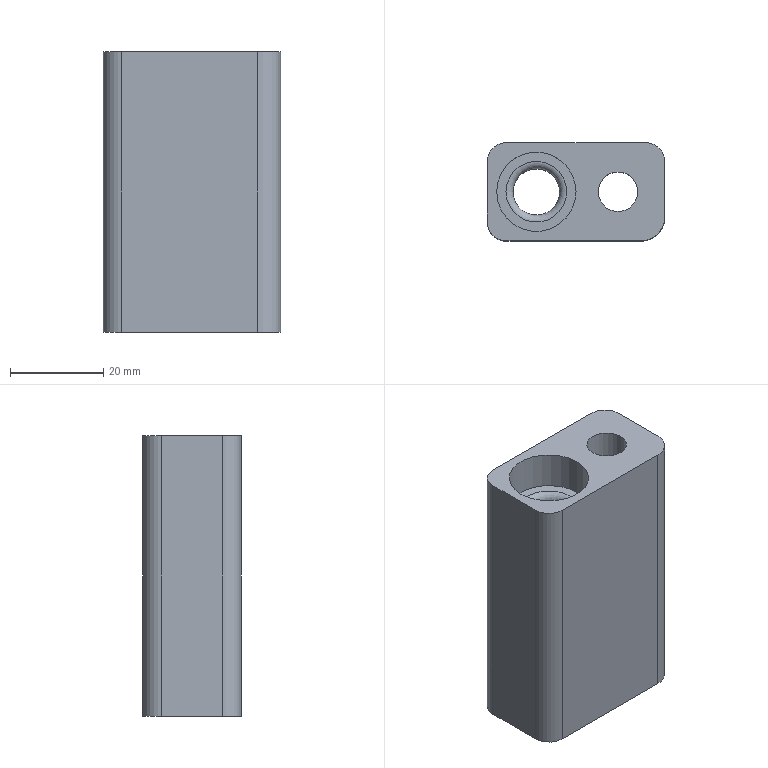Part | STEP file | gslz 2016.10.28-10_id2338_x_t | 1 solid | 17 faces | box 38 x 21 x 60 mm | volume 33724 mm3 | plane 8 | cylinder 8 | torus 1 | commonest cylinder face diameters 8 x3 10 x2 8.5 x1 14 x1 17 x1
STEP:
#1=CARTESIAN_POINT('',(0.,0.,0.));
#2=DIRECTION('',(0.,0.,1.));
#3=DIRECTION('',(1.,0.,0.));
#4=AXIS2_PLACEMENT_3D('',#1,#2,#3);
#5=CARTESIAN_POINT('',(1013.442,-82.206,85.));
#6=VERTEX_POINT('',#5);
#7=CARTESIAN_POINT('',(1021.942,-82.206,85.));
#8=DIRECTION('',(0.,0.,1.));
#9=DIRECTION('',(-1.,0.,0.));
#10=AXIS2_PLACEMENT_3D('',#7,#8,#9);
#11=CIRCLE('',#10,8.5);
#12=CARTESIAN_POINT('',(980.942,-76.206,85.));
#13=DIRECTION('',(0.,0.,1.));
#14=DIRECTION('',(1.,0.,0.));
#15=AXIS2_PLACEMENT_3D('',#12,#13,#14);
#16=PLANE('',#15);
#17=CARTESIAN_POINT('',(41.,-6.));
#18=DIRECTION('',(-1.,0.));
#19=AXIS2_PLACEMENT_2D('',#17,#18);
#20=CIRCLE('',#19,8.5);
#21=(GEOMETRIC_REPRESENTATION_CONTEXT(2)PARAMETRIC_REPRESENTATION_CONTEXT()REPRESENTATION_CONTEXT('',''));
#22=DEFINITIONAL_REPRESENTATION('',(#20),#21);
#23=PCURVE('',#16,#22);
#24=CARTESIAN_POINT('',(1021.942,-82.206,81.));
#25=DIRECTION('',(0.,0.,-1.));
#26=DIRECTION('',(1.,0.,0.));
#27=AXIS2_PLACEMENT_3D('',#24,#25,#26);
#28=CYLINDRICAL_SURFACE('',#27,8.5);
#29=CARTESIAN_POINT('',(9.425,-4.));
#30=DIRECTION('',(-1.,0.));
#31=VECTOR('',#30,1.);
#32=LINE('',#29,#31);
#33=(GEOMETRIC_REPRESENTATION_CONTEXT(2)PARAMETRIC_REPRESENTATION_CONTEXT()REPRESENTATION_CONTEXT('',''));
#34=DEFINITIONAL_REPRESENTATION('',(#32),#33);
#35=PCURVE('',#28,#34);
#36=SURFACE_CURVE('',#11,(#23,#35),.PCURVE_S1.);
#37=EDGE_CURVE('',#6,#6,#36,.T.);
#38=ORIENTED_EDGE('',*,*,#37,.F.);
#39=EDGE_LOOP('',(#38));
#40=FACE_BOUND('',#39,.T.);
#41=CARTESIAN_POINT('',(1049.442,-87.706,85.));
#42=VERTEX_POINT('',#41);
#43=CARTESIAN_POINT('',(1049.442,-75.706,85.));
#44=VERTEX_POINT('',#43);
#45=CARTESIAN_POINT('',(1049.442,-76.206,85.));
#46=DIRECTION('',(0.,1.,0.));
#47=VECTOR('',#46,1.);
#48=LINE('',#45,#47);
#49=CARTESIAN_POINT('',(68.5,0.));
#50=DIRECTION('',(0.,1.));
#51=VECTOR('',#50,1.);
#52=LINE('',#49,#51);
#53=(GEOMETRIC_REPRESENTATION_CONTEXT(2)PARAMETRIC_REPRESENTATION_CONTEXT()REPRESENTATION_CONTEXT('',''));
#54=DEFINITIONAL_REPRESENTATION('',(#52),#53);
#55=PCURVE('',#16,#54);
#56=CARTESIAN_POINT('',(1049.442,-82.206,43.5));
#57=DIRECTION('',(1.,0.,0.));
#58=DIRECTION('',(0.,0.,-1.));
#59=AXIS2_PLACEMENT_3D('',#56,#57,#58);
#60=PLANE('',#59);
#61=CARTESIAN_POINT('',(-41.5,6.));
#62=DIRECTION('',(0.,1.));
#63=VECTOR('',#62,1.);
#64=LINE('',#61,#63);
#65=(GEOMETRIC_REPRESENTATION_CONTEXT(2)PARAMETRIC_REPRESENTATION_CONTEXT()REPRESENTATION_CONTEXT('',''));
#66=DEFINITIONAL_REPRESENTATION('',(#64),#65);
#67=PCURVE('',#60,#66);
#68=SURFACE_CURVE('',#48,(#55,#67),.PCURVE_S1.);
#69=EDGE_CURVE('',#42,#44,#68,.T.);
#70=ORIENTED_EDGE('',*,*,#69,.T.);
#71=CARTESIAN_POINT('',(1045.442,-71.706,85.));
#72=VERTEX_POINT('',#71);
#73=CARTESIAN_POINT('',(1045.442,-75.706,85.));
#74=DIRECTION('',(0.,0.,1.));
#75=DIRECTION('',(-1.,0.,0.));
#76=AXIS2_PLACEMENT_3D('',#73,#74,#75);
#77=CIRCLE('',#76,4.);
#78=CARTESIAN_POINT('',(64.5,0.5));
#79=DIRECTION('',(-1.,0.));
#80=AXIS2_PLACEMENT_2D('',#78,#79);
#81=CIRCLE('',#80,4.);
#82=(GEOMETRIC_REPRESENTATION_CONTEXT(2)PARAMETRIC_REPRESENTATION_CONTEXT()REPRESENTATION_CONTEXT('',''));
#83=DEFINITIONAL_REPRESENTATION('',(#81),#82);
#84=PCURVE('',#16,#83);
#85=CARTESIAN_POINT('',(1045.442,-75.706,43.5));
#86=DIRECTION('',(0.,0.,-1.));
#87=DIRECTION('',(-1.,0.,0.));
#88=AXIS2_PLACEMENT_3D('',#85,#86,#87);
#89=CYLINDRICAL_SURFACE('',#88,4.);
#90=CARTESIAN_POINT('',(6.283,-41.5));
#91=DIRECTION('',(-1.,0.));
#92=VECTOR('',#91,1.);
#93=LINE('',#90,#92);
#94=(GEOMETRIC_REPRESENTATION_CONTEXT(2)PARAMETRIC_REPRESENTATION_CONTEXT()REPRESENTATION_CONTEXT('',''));
#95=DEFINITIONAL_REPRESENTATION('',(#93),#94);
#96=PCURVE('',#89,#95);
#97=SURFACE_CURVE('',#77,(#84,#96),.PCURVE_S1.);
#98=EDGE_CURVE('',#44,#72,#97,.T.);
#99=ORIENTED_EDGE('',*,*,#98,.T.);
#100=CARTESIAN_POINT('',(1015.442,-71.706,85.));
#101=VERTEX_POINT('',#100);
#102=CARTESIAN_POINT('',(938.307,-71.706,85.));
#103=DIRECTION('',(-1.,0.,0.));
#104=VECTOR('',#103,1.);
#105=LINE('',#102,#104);
#106=CARTESIAN_POINT('',(-42.635,4.5));
#107=DIRECTION('',(-1.,0.));
#108=VECTOR('',#107,1.);
#109=LINE('',#106,#108);
#110=(GEOMETRIC_REPRESENTATION_CONTEXT(2)PARAMETRIC_REPRESENTATION_CONTEXT()REPRESENTATION_CONTEXT('',''));
#111=DEFINITIONAL_REPRESENTATION('',(#109),#110);
#112=PCURVE('',#16,#111);
#113=CARTESIAN_POINT('',(938.307,-71.706,80.));
#114=DIRECTION('',(0.,-1.,0.));
#115=DIRECTION('',(0.,0.,-1.));
#116=AXIS2_PLACEMENT_3D('',#113,#114,#115);
#117=PLANE('',#116);
#118=CARTESIAN_POINT('',(-5.,0.));
#119=DIRECTION('',(0.,-1.));
#120=VECTOR('',#119,1.);
#121=LINE('',#118,#120);
#122=(GEOMETRIC_REPRESENTATION_CONTEXT(2)PARAMETRIC_REPRESENTATION_CONTEXT()REPRESENTATION_CONTEXT('',''));
#123=DEFINITIONAL_REPRESENTATION('',(#121),#122);
#124=PCURVE('',#117,#123);
#125=SURFACE_CURVE('',#105,(#112,#124),.PCURVE_S1.);
#126=EDGE_CURVE('',#72,#101,#125,.T.);
#127=ORIENTED_EDGE('',*,*,#126,.T.);
#128=CARTESIAN_POINT('',(1011.442,-75.706,85.));
#129=VERTEX_POINT('',#128);
#130=CARTESIAN_POINT('',(1015.442,-75.706,85.));
#131=DIRECTION('',(0.,0.,1.));
#132=DIRECTION('',(-1.,0.,0.));
#133=AXIS2_PLACEMENT_3D('',#130,#131,#132);
#134=CIRCLE('',#133,4.);
#135=CARTESIAN_POINT('',(34.5,0.5));
#136=DIRECTION('',(-1.,0.));
#137=AXIS2_PLACEMENT_2D('',#135,#136);
#138=CIRCLE('',#137,4.);
#139=(GEOMETRIC_REPRESENTATION_CONTEXT(2)PARAMETRIC_REPRESENTATION_CONTEXT()REPRESENTATION_CONTEXT('',''));
#140=DEFINITIONAL_REPRESENTATION('',(#138),#139);
#141=PCURVE('',#16,#140);
#142=CARTESIAN_POINT('',(1015.442,-75.706,46.));
#143=DIRECTION('',(0.,0.,-1.));
#144=DIRECTION('',(-1.,0.,0.));
#145=AXIS2_PLACEMENT_3D('',#142,#143,#144);
#146=CYLINDRICAL_SURFACE('',#145,4.);
#147=CARTESIAN_POINT('',(6.283,-39.));
#148=DIRECTION('',(-1.,0.));
#149=VECTOR('',#148,1.);
#150=LINE('',#147,#149);
#151=(GEOMETRIC_REPRESENTATION_CONTEXT(2)PARAMETRIC_REPRESENTATION_CONTEXT()REPRESENTATION_CONTEXT('',''));
#152=DEFINITIONAL_REPRESENTATION('',(#150),#151);
#153=PCURVE('',#146,#152);
#154=SURFACE_CURVE('',#134,(#141,#153),.PCURVE_S1.);
#155=EDGE_CURVE('',#101,#129,#154,.T.);
#156=ORIENTED_EDGE('',*,*,#155,.T.);
#157=CARTESIAN_POINT('',(1011.442,-88.706,85.));
#158=VERTEX_POINT('',#157);
#159=CARTESIAN_POINT('',(1011.442,-82.206,85.));
#160=DIRECTION('',(0.,-1.,0.));
#161=VECTOR('',#160,1.);
#162=LINE('',#159,#161);
#163=CARTESIAN_POINT('',(30.5,-6.));
#164=DIRECTION('',(0.,-1.));
#165=VECTOR('',#164,1.);
#166=LINE('',#163,#165);
#167=(GEOMETRIC_REPRESENTATION_CONTEXT(2)PARAMETRIC_REPRESENTATION_CONTEXT()REPRESENTATION_CONTEXT('',''));
#168=DEFINITIONAL_REPRESENTATION('',(#166),#167);
#169=PCURVE('',#16,#168);
#170=CARTESIAN_POINT('',(1011.442,-82.206,46.));
#171=DIRECTION('',(1.,0.,0.));
#172=DIRECTION('',(0.,0.,-1.));
#173=AXIS2_PLACEMENT_3D('',#170,#171,#172);
#174=PLANE('',#173);
#175=CARTESIAN_POINT('',(-39.,0.));
#176=DIRECTION('',(0.,-1.));
#177=VECTOR('',#176,1.);
#178=LINE('',#175,#177);
#179=(GEOMETRIC_REPRESENTATION_CONTEXT(2)PARAMETRIC_REPRESENTATION_CONTEXT()REPRESENTATION_CONTEXT('',''));
#180=DEFINITIONAL_REPRESENTATION('',(#178),#179);
#181=PCURVE('',#174,#180);
#182=SURFACE_CURVE('',#162,(#169,#181),.PCURVE_S1.);
#183=EDGE_CURVE('',#129,#158,#182,.T.);
#184=ORIENTED_EDGE('',*,*,#183,.T.);
#185=CARTESIAN_POINT('',(1015.442,-92.706,85.));
#186=VERTEX_POINT('',#185);
#187=CARTESIAN_POINT('',(1015.442,-88.706,85.));
#188=DIRECTION('',(0.,0.,1.));
#189=DIRECTION('',(-1.,0.,0.));
#190=AXIS2_PLACEMENT_3D('',#187,#188,#189);
#191=CIRCLE('',#190,4.);
#192=CARTESIAN_POINT('',(34.5,-12.5));
#193=DIRECTION('',(-1.,0.));
#194=AXIS2_PLACEMENT_2D('',#192,#193);
#195=CIRCLE('',#194,4.);
#196=(GEOMETRIC_REPRESENTATION_CONTEXT(2)PARAMETRIC_REPRESENTATION_CONTEXT()REPRESENTATION_CONTEXT('',''));
#197=DEFINITIONAL_REPRESENTATION('',(#195),#196);
#198=PCURVE('',#16,#197);
#199=CARTESIAN_POINT('',(1015.442,-88.706,80.));
#200=DIRECTION('',(0.,0.,-1.));
#201=DIRECTION('',(-1.,0.,0.));
#202=AXIS2_PLACEMENT_3D('',#199,#200,#201);
#203=CYLINDRICAL_SURFACE('',#202,4.);
#204=CARTESIAN_POINT('',(6.283,-5.));
#205=DIRECTION('',(-1.,0.));
#206=VECTOR('',#205,1.);
#207=LINE('',#204,#206);
#208=(GEOMETRIC_REPRESENTATION_CONTEXT(2)PARAMETRIC_REPRESENTATION_CONTEXT()REPRESENTATION_CONTEXT('',''));
#209=DEFINITIONAL_REPRESENTATION('',(#207),#208);
#210=PCURVE('',#203,#209);
#211=SURFACE_CURVE('',#191,(#198,#210),.PCURVE_S1.);
#212=EDGE_CURVE('',#158,#186,#211,.T.);
#213=ORIENTED_EDGE('',*,*,#212,.T.);
#214=CARTESIAN_POINT('',(1044.442,-92.706,85.));
#215=VERTEX_POINT('',#214);
#216=CARTESIAN_POINT('',(1673.942,-92.706,85.));
#217=DIRECTION('',(1.,0.,0.));
#218=VECTOR('',#217,1.);
#219=LINE('',#216,#218);
#220=CARTESIAN_POINT('',(693.,-16.5));
#221=DIRECTION('',(1.,0.));
#222=VECTOR('',#221,1.);
#223=LINE('',#220,#222);
#224=(GEOMETRIC_REPRESENTATION_CONTEXT(2)PARAMETRIC_REPRESENTATION_CONTEXT()REPRESENTATION_CONTEXT('',''));
#225=DEFINITIONAL_REPRESENTATION('',(#223),#224);
#226=PCURVE('',#16,#225);
#227=CARTESIAN_POINT('',(1673.942,-92.706,80.));
#228=DIRECTION('',(0.,1.,0.));
#229=DIRECTION('',(0.,0.,1.));
#230=AXIS2_PLACEMENT_3D('',#227,#228,#229);
#231=PLANE('',#230);
#232=CARTESIAN_POINT('',(5.,0.));
#233=DIRECTION('',(0.,1.));
#234=VECTOR('',#233,1.);
#235=LINE('',#232,#234);
#236=(GEOMETRIC_REPRESENTATION_CONTEXT(2)PARAMETRIC_REPRESENTATION_CONTEXT()REPRESENTATION_CONTEXT('',''));
#237=DEFINITIONAL_REPRESENTATION('',(#235),#236);
#238=PCURVE('',#231,#237);
#239=SURFACE_CURVE('',#219,(#226,#238),.PCURVE_S1.);
#240=EDGE_CURVE('',#186,#215,#239,.T.);
#241=ORIENTED_EDGE('',*,*,#240,.T.);
#242=CARTESIAN_POINT('',(1044.442,-87.706,85.));
#243=DIRECTION('',(0.,0.,1.));
#244=DIRECTION('',(-1.,0.,0.));
#245=AXIS2_PLACEMENT_3D('',#242,#243,#244);
#246=CIRCLE('',#245,5.);
#247=CARTESIAN_POINT('',(63.5,-11.5));
#248=DIRECTION('',(-1.,0.));
#249=AXIS2_PLACEMENT_2D('',#247,#248);
#250=CIRCLE('',#249,5.);
#251=(GEOMETRIC_REPRESENTATION_CONTEXT(2)PARAMETRIC_REPRESENTATION_CONTEXT()REPRESENTATION_CONTEXT('',''));
#252=DEFINITIONAL_REPRESENTATION('',(#250),#251);
#253=PCURVE('',#16,#252);
#254=CARTESIAN_POINT('',(1044.442,-87.706,43.5));
#255=DIRECTION('',(0.,0.,1.));
#256=DIRECTION('',(1.,0.,0.));
#257=AXIS2_PLACEMENT_3D('',#254,#255,#256);
#258=CYLINDRICAL_SURFACE('',#257,5.);
#259=CARTESIAN_POINT('',(3.142,41.5));
#260=DIRECTION('',(1.,0.));
#261=VECTOR('',#260,1.);
#262=LINE('',#259,#261);
#263=(GEOMETRIC_REPRESENTATION_CONTEXT(2)PARAMETRIC_REPRESENTATION_CONTEXT()REPRESENTATION_CONTEXT('',''));
#264=DEFINITIONAL_REPRESENTATION('',(#262),#263);
#265=PCURVE('',#258,#264);
#266=SURFACE_CURVE('',#246,(#253,#265),.PCURVE_S1.);
#267=EDGE_CURVE('',#215,#42,#266,.T.);
#268=ORIENTED_EDGE('',*,*,#267,.T.);
#269=EDGE_LOOP('',(#70,#99,#127,#156,#184,#213,#241,#268));
#270=FACE_BOUND('',#269,.T.);
#271=CARTESIAN_POINT('',(1035.192,-82.206,85.));
#272=VERTEX_POINT('',#271);
#273=CARTESIAN_POINT('',(1039.442,-82.206,85.));
#274=DIRECTION('',(0.,0.,-1.));
#275=DIRECTION('',(-1.,0.,0.));
#276=AXIS2_PLACEMENT_3D('',#273,#274,#275);
#277=CIRCLE('',#276,4.25);
#278=CARTESIAN_POINT('',(54.25,-6.));
#279=CARTESIAN_POINT('',(54.25,1.361));
#280=CARTESIAN_POINT('',(60.625,-2.319));
#281=CARTESIAN_POINT('',(67.,-6.));
#282=CARTESIAN_POINT('',(60.625,-9.681));
#283=CARTESIAN_POINT('',(54.25,-13.361));
#284=CARTESIAN_POINT('',(54.25,-6.));
#285=(BOUNDED_CURVE()B_SPLINE_CURVE(2,(#278,#279,#280,#281,#282,#283,#284),.UNSPECIFIED.,.T.,.F.)B_SPLINE_CURVE_WITH_KNOTS((1,2,2,2,2,1),(-2.094,0.,2.094,4.189,6.283,8.378),.UNSPECIFIED.)CURVE()GEOMETRIC_REPRESENTATION_ITEM()RATIONAL_B_SPLINE_CURVE((1.,0.5,1.,0.5,1.,0.5,1.))REPRESENTATION_ITEM(''));
#286=(GEOMETRIC_REPRESENTATION_CONTEXT(2)PARAMETRIC_REPRESENTATION_CONTEXT()REPRESENTATION_CONTEXT('',''));
#287=DEFINITIONAL_REPRESENTATION('',(#285),#286);
#288=PCURVE('',#16,#287);
#289=CARTESIAN_POINT('',(1039.442,-82.206,-18.));
#290=DIRECTION('',(0.,0.,1.));
#291=DIRECTION('',(1.,0.,0.));
#292=AXIS2_PLACEMENT_3D('',#289,#290,#291);
#293=CYLINDRICAL_SURFACE('',#292,4.25);
#294=CARTESIAN_POINT('',(9.425,103.));
#295=DIRECTION('',(-1.,0.));
#296=VECTOR('',#295,1.);
#297=LINE('',#294,#296);
#298=(GEOMETRIC_REPRESENTATION_CONTEXT(2)PARAMETRIC_REPRESENTATION_CONTEXT()REPRESENTATION_CONTEXT('',''));
#299=DEFINITIONAL_REPRESENTATION('',(#297),#298);
#300=PCURVE('',#293,#299);
#301=SURFACE_CURVE('',#277,(#288,#300),.PCURVE_S1.);
#302=EDGE_CURVE('',#272,#272,#301,.T.);
#303=ORIENTED_EDGE('',*,*,#302,.T.);
#304=EDGE_LOOP('',(#303));
#305=FACE_BOUND('',#304,.T.);
#306=ADVANCED_FACE('',(#40,#270,#305),#16,.T.);
#307=CARTESIAN_POINT('',(1016.942,-82.206,25.));
#308=VERTEX_POINT('',#307);
#309=CARTESIAN_POINT('',(1021.942,-82.206,25.));
#310=DIRECTION('',(0.,0.,1.));
#311=DIRECTION('',(-1.,0.,0.));
#312=AXIS2_PLACEMENT_3D('',#309,#310,#311);
#313=CIRCLE('',#312,5.);
#314=CARTESIAN_POINT('',(972.942,-136.206,25.));
#315=DIRECTION('',(0.,0.,-1.));
#316=DIRECTION('',(-1.,0.,0.));
#317=AXIS2_PLACEMENT_3D('',#314,#315,#316);
#318=PLANE('',#317);
#319=CARTESIAN_POINT('',(-44.,54.));
#320=CARTESIAN_POINT('',(-44.,45.34));
#321=CARTESIAN_POINT('',(-51.5,49.67));
#322=CARTESIAN_POINT('',(-59.,54.));
#323=CARTESIAN_POINT('',(-51.5,58.33));
#324=CARTESIAN_POINT('',(-44.,62.66));
#325=CARTESIAN_POINT('',(-44.,54.));
#326=(BOUNDED_CURVE()B_SPLINE_CURVE(2,(#319,#320,#321,#322,#323,#324,#325),.UNSPECIFIED.,.T.,.F.)B_SPLINE_CURVE_WITH_KNOTS((1,2,2,2,2,1),(-2.094,0.,2.094,4.189,6.283,8.378),.UNSPECIFIED.)CURVE()GEOMETRIC_REPRESENTATION_ITEM()RATIONAL_B_SPLINE_CURVE((1.,0.5,1.,0.5,1.,0.5,1.))REPRESENTATION_ITEM(''));
#327=(GEOMETRIC_REPRESENTATION_CONTEXT(2)PARAMETRIC_REPRESENTATION_CONTEXT()REPRESENTATION_CONTEXT('',''));
#328=DEFINITIONAL_REPRESENTATION('',(#326),#327);
#329=PCURVE('',#318,#328);
#330=CARTESIAN_POINT('',(1021.942,-82.206,45.5));
#331=DIRECTION('',(0.,0.,-1.));
#332=DIRECTION('',(1.,0.,0.));
#333=AXIS2_PLACEMENT_3D('',#330,#331,#332);
#334=CYLINDRICAL_SURFACE('',#333,5.);
#335=CARTESIAN_POINT('',(9.425,20.5));
#336=DIRECTION('',(-1.,0.));
#337=VECTOR('',#336,1.);
#338=LINE('',#335,#337);
#339=(GEOMETRIC_REPRESENTATION_CONTEXT(2)PARAMETRIC_REPRESENTATION_CONTEXT()REPRESENTATION_CONTEXT('',''));
#340=DEFINITIONAL_REPRESENTATION('',(#338),#339);
#341=PCURVE('',#334,#340);
#342=SURFACE_CURVE('',#313,(#329,#341),.PCURVE_S1.);
#343=EDGE_CURVE('',#308,#308,#342,.T.);
#344=ORIENTED_EDGE('',*,*,#343,.T.);
#345=EDGE_LOOP('',(#344));
#346=FACE_BOUND('',#345,.T.);
#347=CARTESIAN_POINT('',(1032.442,-82.206,25.));
#348=VERTEX_POINT('',#347);
#349=CARTESIAN_POINT('',(1039.442,-82.206,25.));
#350=DIRECTION('',(0.,0.,1.));
#351=DIRECTION('',(-1.,0.,0.));
#352=AXIS2_PLACEMENT_3D('',#349,#350,#351);
#353=CIRCLE('',#352,7.);
#354=CARTESIAN_POINT('',(-59.5,54.));
#355=CARTESIAN_POINT('',(-59.5,41.876));
#356=CARTESIAN_POINT('',(-70.,47.938));
#357=CARTESIAN_POINT('',(-80.5,54.));
#358=CARTESIAN_POINT('',(-70.,60.062));
#359=CARTESIAN_POINT('',(-59.5,66.124));
#360=CARTESIAN_POINT('',(-59.5,54.));
#361=(BOUNDED_CURVE()B_SPLINE_CURVE(2,(#354,#355,#356,#357,#358,#359,#360),.UNSPECIFIED.,.T.,.F.)B_SPLINE_CURVE_WITH_KNOTS((1,2,2,2,2,1),(-2.094,0.,2.094,4.189,6.283,8.378),.UNSPECIFIED.)CURVE()GEOMETRIC_REPRESENTATION_ITEM()RATIONAL_B_SPLINE_CURVE((1.,0.5,1.,0.5,1.,0.5,1.))REPRESENTATION_ITEM(''));
#362=(GEOMETRIC_REPRESENTATION_CONTEXT(2)PARAMETRIC_REPRESENTATION_CONTEXT()REPRESENTATION_CONTEXT('',''));
#363=DEFINITIONAL_REPRESENTATION('',(#361),#362);
#364=PCURVE('',#318,#363);
#365=CARTESIAN_POINT('',(1039.442,-82.206,-8.));
#366=DIRECTION('',(0.,0.,1.));
#367=DIRECTION('',(1.,0.,0.));
#368=AXIS2_PLACEMENT_3D('',#365,#366,#367);
#369=CYLINDRICAL_SURFACE('',#368,7.);
#370=CARTESIAN_POINT('',(3.142,33.));
#371=DIRECTION('',(1.,0.));
#372=VECTOR('',#371,1.);
#373=LINE('',#370,#372);
#374=(GEOMETRIC_REPRESENTATION_CONTEXT(2)PARAMETRIC_REPRESENTATION_CONTEXT()REPRESENTATION_CONTEXT('',''));
#375=DEFINITIONAL_REPRESENTATION('',(#373),#374);
#376=PCURVE('',#369,#375);
#377=SURFACE_CURVE('',#353,(#364,#376),.PCURVE_S1.);
#378=EDGE_CURVE('',#348,#348,#377,.T.);
#379=ORIENTED_EDGE('',*,*,#378,.T.);
#380=EDGE_LOOP('',(#379));
#381=FACE_BOUND('',#380,.T.);
#382=CARTESIAN_POINT('',(1045.442,-71.706,25.));
#383=VERTEX_POINT('',#382);
#384=CARTESIAN_POINT('',(1015.442,-71.706,25.));
#385=VERTEX_POINT('',#384);
#386=CARTESIAN_POINT('',(972.942,-71.706,25.));
#387=DIRECTION('',(-1.,0.,0.));
#388=VECTOR('',#387,1.);
#389=LINE('',#386,#388);
#390=CARTESIAN_POINT('',(0.,64.5));
#391=DIRECTION('',(1.,0.));
#392=VECTOR('',#391,1.);
#393=LINE('',#390,#392);
#394=(GEOMETRIC_REPRESENTATION_CONTEXT(2)PARAMETRIC_REPRESENTATION_CONTEXT()REPRESENTATION_CONTEXT('',''));
#395=DEFINITIONAL_REPRESENTATION('',(#393),#394);
#396=PCURVE('',#318,#395);
#397=CARTESIAN_POINT('',(55.,34.635));
#398=DIRECTION('',(0.,-1.));
#399=VECTOR('',#398,1.);
#400=LINE('',#397,#399);
#401=(GEOMETRIC_REPRESENTATION_CONTEXT(2)PARAMETRIC_REPRESENTATION_CONTEXT()REPRESENTATION_CONTEXT('',''));
#402=DEFINITIONAL_REPRESENTATION('',(#400),#401);
#403=PCURVE('',#117,#402);
#404=SURFACE_CURVE('',#389,(#396,#403),.PCURVE_S1.);
#405=EDGE_CURVE('',#383,#385,#404,.T.);
#406=ORIENTED_EDGE('',*,*,#405,.F.);
#407=CARTESIAN_POINT('',(1049.442,-75.706,25.));
#408=VERTEX_POINT('',#407);
#409=CARTESIAN_POINT('',(1045.442,-75.706,25.));
#410=DIRECTION('',(0.,0.,-1.));
#411=DIRECTION('',(-1.,0.,0.));
#412=AXIS2_PLACEMENT_3D('',#409,#410,#411);
#413=CIRCLE('',#412,4.);
#414=CARTESIAN_POINT('',(-72.5,60.5));
#415=DIRECTION('',(1.,0.));
#416=AXIS2_PLACEMENT_2D('',#414,#415);
#417=CIRCLE('',#416,4.);
#418=(GEOMETRIC_REPRESENTATION_CONTEXT(2)PARAMETRIC_REPRESENTATION_CONTEXT()REPRESENTATION_CONTEXT('',''));
#419=DEFINITIONAL_REPRESENTATION('',(#417),#418);
#420=PCURVE('',#318,#419);
#421=CARTESIAN_POINT('',(0.,18.5));
#422=DIRECTION('',(1.,0.));
#423=VECTOR('',#422,1.);
#424=LINE('',#421,#423);
#425=(GEOMETRIC_REPRESENTATION_CONTEXT(2)PARAMETRIC_REPRESENTATION_CONTEXT()REPRESENTATION_CONTEXT('',''));
#426=DEFINITIONAL_REPRESENTATION('',(#424),#425);
#427=PCURVE('',#89,#426);
#428=SURFACE_CURVE('',#413,(#420,#427),.PCURVE_S1.);
#429=EDGE_CURVE('',#383,#408,#428,.T.);
#430=ORIENTED_EDGE('',*,*,#429,.T.);
#431=CARTESIAN_POINT('',(1049.442,-87.706,25.));
#432=VERTEX_POINT('',#431);
#433=CARTESIAN_POINT('',(1049.442,-136.206,25.));
#434=DIRECTION('',(0.,-1.,0.));
#435=VECTOR('',#434,1.);
#436=LINE('',#433,#435);
#437=CARTESIAN_POINT('',(-76.5,0.));
#438=DIRECTION('',(0.,-1.));
#439=VECTOR('',#438,1.);
#440=LINE('',#437,#439);
#441=(GEOMETRIC_REPRESENTATION_CONTEXT(2)PARAMETRIC_REPRESENTATION_CONTEXT()REPRESENTATION_CONTEXT('',''));
#442=DEFINITIONAL_REPRESENTATION('',(#440),#441);
#443=PCURVE('',#318,#442);
#444=CARTESIAN_POINT('',(18.5,-54.));
#445=DIRECTION('',(0.,-1.));
#446=VECTOR('',#445,1.);
#447=LINE('',#444,#446);
#448=(GEOMETRIC_REPRESENTATION_CONTEXT(2)PARAMETRIC_REPRESENTATION_CONTEXT()REPRESENTATION_CONTEXT('',''));
#449=DEFINITIONAL_REPRESENTATION('',(#447),#448);
#450=PCURVE('',#60,#449);
#451=SURFACE_CURVE('',#436,(#443,#450),.PCURVE_S1.);
#452=EDGE_CURVE('',#408,#432,#451,.T.);
#453=ORIENTED_EDGE('',*,*,#452,.T.);
#454=CARTESIAN_POINT('',(1044.442,-92.706,25.));
#455=VERTEX_POINT('',#454);
#456=CARTESIAN_POINT('',(1044.442,-87.706,25.));
#457=DIRECTION('',(0.,0.,-1.));
#458=DIRECTION('',(-1.,0.,0.));
#459=AXIS2_PLACEMENT_3D('',#456,#457,#458);
#460=CIRCLE('',#459,5.);
#461=CARTESIAN_POINT('',(-71.5,48.5));
#462=DIRECTION('',(1.,0.));
#463=AXIS2_PLACEMENT_2D('',#461,#462);
#464=CIRCLE('',#463,5.);
#465=(GEOMETRIC_REPRESENTATION_CONTEXT(2)PARAMETRIC_REPRESENTATION_CONTEXT()REPRESENTATION_CONTEXT('',''));
#466=DEFINITIONAL_REPRESENTATION('',(#464),#465);
#467=PCURVE('',#318,#466);
#468=CARTESIAN_POINT('',(9.425,-18.5));
#469=DIRECTION('',(-1.,0.));
#470=VECTOR('',#469,1.);
#471=LINE('',#468,#470);
#472=(GEOMETRIC_REPRESENTATION_CONTEXT(2)PARAMETRIC_REPRESENTATION_CONTEXT()REPRESENTATION_CONTEXT('',''));
#473=DEFINITIONAL_REPRESENTATION('',(#471),#472);
#474=PCURVE('',#258,#473);
#475=SURFACE_CURVE('',#460,(#467,#474),.PCURVE_S1.);
#476=EDGE_CURVE('',#432,#455,#475,.T.);
#477=ORIENTED_EDGE('',*,*,#476,.T.);
#478=CARTESIAN_POINT('',(1015.442,-92.706,25.));
#479=VERTEX_POINT('',#478);
#480=CARTESIAN_POINT('',(972.942,-92.706,25.));
#481=DIRECTION('',(1.,0.,0.));
#482=VECTOR('',#481,1.);
#483=LINE('',#480,#482);
#484=CARTESIAN_POINT('',(0.,43.5));
#485=DIRECTION('',(-1.,0.));
#486=VECTOR('',#485,1.);
#487=LINE('',#484,#486);
#488=(GEOMETRIC_REPRESENTATION_CONTEXT(2)PARAMETRIC_REPRESENTATION_CONTEXT()REPRESENTATION_CONTEXT('',''));
#489=DEFINITIONAL_REPRESENTATION('',(#487),#488);
#490=PCURVE('',#318,#489);
#491=CARTESIAN_POINT('',(-55.,-701.));
#492=DIRECTION('',(0.,1.));
#493=VECTOR('',#492,1.);
#494=LINE('',#491,#493);
#495=(GEOMETRIC_REPRESENTATION_CONTEXT(2)PARAMETRIC_REPRESENTATION_CONTEXT()REPRESENTATION_CONTEXT('',''));
#496=DEFINITIONAL_REPRESENTATION('',(#494),#495);
#497=PCURVE('',#231,#496);
#498=SURFACE_CURVE('',#483,(#490,#497),.PCURVE_S1.);
#499=EDGE_CURVE('',#479,#455,#498,.T.);
#500=ORIENTED_EDGE('',*,*,#499,.F.);
#501=CARTESIAN_POINT('',(1011.442,-88.706,25.));
#502=VERTEX_POINT('',#501);
#503=CARTESIAN_POINT('',(1015.442,-88.706,25.));
#504=DIRECTION('',(0.,0.,-1.));
#505=DIRECTION('',(-1.,0.,0.));
#506=AXIS2_PLACEMENT_3D('',#503,#504,#505);
#507=CIRCLE('',#506,4.);
#508=CARTESIAN_POINT('',(-42.5,47.5));
#509=DIRECTION('',(1.,0.));
#510=AXIS2_PLACEMENT_2D('',#508,#509);
#511=CIRCLE('',#510,4.);
#512=(GEOMETRIC_REPRESENTATION_CONTEXT(2)PARAMETRIC_REPRESENTATION_CONTEXT()REPRESENTATION_CONTEXT('',''));
#513=DEFINITIONAL_REPRESENTATION('',(#511),#512);
#514=PCURVE('',#318,#513);
#515=CARTESIAN_POINT('',(0.,55.));
#516=DIRECTION('',(1.,0.));
#517=VECTOR('',#516,1.);
#518=LINE('',#515,#517);
#519=(GEOMETRIC_REPRESENTATION_CONTEXT(2)PARAMETRIC_REPRESENTATION_CONTEXT()REPRESENTATION_CONTEXT('',''));
#520=DEFINITIONAL_REPRESENTATION('',(#518),#519);
#521=PCURVE('',#203,#520);
#522=SURFACE_CURVE('',#507,(#514,#521),.PCURVE_S1.);
#523=EDGE_CURVE('',#479,#502,#522,.T.);
#524=ORIENTED_EDGE('',*,*,#523,.T.);
#525=CARTESIAN_POINT('',(1011.442,-75.706,25.));
#526=VERTEX_POINT('',#525);
#527=CARTESIAN_POINT('',(1011.442,-82.206,25.));
#528=DIRECTION('',(0.,1.,0.));
#529=VECTOR('',#528,1.);
#530=LINE('',#527,#529);
#531=CARTESIAN_POINT('',(-38.5,54.));
#532=DIRECTION('',(0.,1.));
#533=VECTOR('',#532,1.);
#534=LINE('',#531,#533);
#535=(GEOMETRIC_REPRESENTATION_CONTEXT(2)PARAMETRIC_REPRESENTATION_CONTEXT()REPRESENTATION_CONTEXT('',''));
#536=DEFINITIONAL_REPRESENTATION('',(#534),#535);
#537=PCURVE('',#318,#536);
#538=CARTESIAN_POINT('',(21.,0.));
#539=DIRECTION('',(0.,1.));
#540=VECTOR('',#539,1.);
#541=LINE('',#538,#540);
#542=(GEOMETRIC_REPRESENTATION_CONTEXT(2)PARAMETRIC_REPRESENTATION_CONTEXT()REPRESENTATION_CONTEXT('',''));
#543=DEFINITIONAL_REPRESENTATION('',(#541),#542);
#544=PCURVE('',#174,#543);
#545=SURFACE_CURVE('',#530,(#537,#544),.PCURVE_S1.);
#546=EDGE_CURVE('',#502,#526,#545,.T.);
#547=ORIENTED_EDGE('',*,*,#546,.T.);
#548=CARTESIAN_POINT('',(1015.442,-75.706,25.));
#549=DIRECTION('',(0.,0.,-1.));
#550=DIRECTION('',(-1.,0.,0.));
#551=AXIS2_PLACEMENT_3D('',#548,#549,#550);
#552=CIRCLE('',#551,4.);
#553=CARTESIAN_POINT('',(-42.5,60.5));
#554=DIRECTION('',(1.,0.));
#555=AXIS2_PLACEMENT_2D('',#553,#554);
#556=CIRCLE('',#555,4.);
#557=(GEOMETRIC_REPRESENTATION_CONTEXT(2)PARAMETRIC_REPRESENTATION_CONTEXT()REPRESENTATION_CONTEXT('',''));
#558=DEFINITIONAL_REPRESENTATION('',(#556),#557);
#559=PCURVE('',#318,#558);
#560=CARTESIAN_POINT('',(0.,21.));
#561=DIRECTION('',(1.,0.));
#562=VECTOR('',#561,1.);
#563=LINE('',#560,#562);
#564=(GEOMETRIC_REPRESENTATION_CONTEXT(2)PARAMETRIC_REPRESENTATION_CONTEXT()REPRESENTATION_CONTEXT('',''));
#565=DEFINITIONAL_REPRESENTATION('',(#563),#564);
#566=PCURVE('',#146,#565);
#567=SURFACE_CURVE('',#552,(#559,#566),.PCURVE_S1.);
#568=EDGE_CURVE('',#526,#385,#567,.T.);
#569=ORIENTED_EDGE('',*,*,#568,.T.);
#570=EDGE_LOOP('',(#406,#430,#453,#477,#500,#524,#547,#569));
#571=FACE_BOUND('',#570,.T.);
#572=ADVANCED_FACE('',(#346,#381,#571),#318,.T.);
#573=ORIENTED_EDGE('',*,*,#499,.T.);
#574=CARTESIAN_POINT('',(1044.442,-92.706,95.));
#575=DIRECTION('',(0.,0.,1.));
#576=VECTOR('',#575,1.);
#577=LINE('',#574,#576);
#578=CARTESIAN_POINT('',(15.,-629.5));
#579=DIRECTION('',(1.,0.));
#580=VECTOR('',#579,1.);
#581=LINE('',#578,#580);
#582=(GEOMETRIC_REPRESENTATION_CONTEXT(2)PARAMETRIC_REPRESENTATION_CONTEXT()REPRESENTATION_CONTEXT('',''));
#583=DEFINITIONAL_REPRESENTATION('',(#581),#582);
#584=PCURVE('',#231,#583);
#585=CARTESIAN_POINT('',(4.712,51.5));
#586=DIRECTION('',(0.,1.));
#587=VECTOR('',#586,1.);
#588=LINE('',#585,#587);
#589=(GEOMETRIC_REPRESENTATION_CONTEXT(2)PARAMETRIC_REPRESENTATION_CONTEXT()REPRESENTATION_CONTEXT('',''));
#590=DEFINITIONAL_REPRESENTATION('',(#588),#589);
#591=PCURVE('',#258,#590);
#592=SURFACE_CURVE('',#577,(#584,#591),.PCURVE_S1.);
#593=EDGE_CURVE('',#455,#215,#592,.T.);
#594=ORIENTED_EDGE('',*,*,#593,.T.);
#595=ORIENTED_EDGE('',*,*,#240,.F.);
#596=CARTESIAN_POINT('',(1015.442,-92.706,80.));
#597=DIRECTION('',(0.,0.,-1.));
#598=VECTOR('',#597,1.);
#599=LINE('',#596,#598);
#600=CARTESIAN_POINT('',(0.,-658.5));
#601=DIRECTION('',(-1.,0.));
#602=VECTOR('',#601,1.);
#603=LINE('',#600,#602);
#604=(GEOMETRIC_REPRESENTATION_CONTEXT(2)PARAMETRIC_REPRESENTATION_CONTEXT()REPRESENTATION_CONTEXT('',''));
#605=DEFINITIONAL_REPRESENTATION('',(#603),#604);
#606=PCURVE('',#231,#605);
#607=CARTESIAN_POINT('',(4.712,0.));
#608=DIRECTION('',(0.,1.));
#609=VECTOR('',#608,1.);
#610=LINE('',#607,#609);
#611=(GEOMETRIC_REPRESENTATION_CONTEXT(2)PARAMETRIC_REPRESENTATION_CONTEXT()REPRESENTATION_CONTEXT('',''));
#612=DEFINITIONAL_REPRESENTATION('',(#610),#611);
#613=PCURVE('',#203,#612);
#614=SURFACE_CURVE('',#599,(#606,#613),.PCURVE_S1.);
#615=EDGE_CURVE('',#186,#479,#614,.T.);
#616=ORIENTED_EDGE('',*,*,#615,.T.);
#617=EDGE_LOOP('',(#573,#594,#595,#616));
#618=FACE_BOUND('',#617,.T.);
#619=ADVANCED_FACE('',(#618),#231,.F.);
#620=ORIENTED_EDGE('',*,*,#126,.F.);
#621=CARTESIAN_POINT('',(1045.442,-71.706,43.5));
#622=DIRECTION('',(0.,0.,-1.));
#623=VECTOR('',#622,1.);
#624=LINE('',#621,#623);
#625=CARTESIAN_POINT('',(36.5,107.135));
#626=DIRECTION('',(1.,0.));
#627=VECTOR('',#626,1.);
#628=LINE('',#625,#627);
#629=(GEOMETRIC_REPRESENTATION_CONTEXT(2)PARAMETRIC_REPRESENTATION_CONTEXT()REPRESENTATION_CONTEXT('',''));
#630=DEFINITIONAL_REPRESENTATION('',(#628),#629);
#631=PCURVE('',#117,#630);
#632=CARTESIAN_POINT('',(1.571,0.));
#633=DIRECTION('',(0.,1.));
#634=VECTOR('',#633,1.);
#635=LINE('',#632,#634);
#636=(GEOMETRIC_REPRESENTATION_CONTEXT(2)PARAMETRIC_REPRESENTATION_CONTEXT()REPRESENTATION_CONTEXT('',''));
#637=DEFINITIONAL_REPRESENTATION('',(#635),#636);
#638=PCURVE('',#89,#637);
#639=SURFACE_CURVE('',#624,(#631,#638),.PCURVE_S1.);
#640=EDGE_CURVE('',#72,#383,#639,.T.);
#641=ORIENTED_EDGE('',*,*,#640,.T.);
#642=ORIENTED_EDGE('',*,*,#405,.T.);
#643=CARTESIAN_POINT('',(1015.442,-71.706,80.));
#644=DIRECTION('',(0.,0.,1.));
#645=VECTOR('',#644,1.);
#646=LINE('',#643,#645);
#647=CARTESIAN_POINT('',(0.,77.135));
#648=DIRECTION('',(-1.,0.));
#649=VECTOR('',#648,1.);
#650=LINE('',#647,#649);
#651=(GEOMETRIC_REPRESENTATION_CONTEXT(2)PARAMETRIC_REPRESENTATION_CONTEXT()REPRESENTATION_CONTEXT('',''));
#652=DEFINITIONAL_REPRESENTATION('',(#650),#651);
#653=PCURVE('',#117,#652);
#654=CARTESIAN_POINT('',(1.571,-34.));
#655=DIRECTION('',(0.,-1.));
#656=VECTOR('',#655,1.);
#657=LINE('',#654,#656);
#658=(GEOMETRIC_REPRESENTATION_CONTEXT(2)PARAMETRIC_REPRESENTATION_CONTEXT()REPRESENTATION_CONTEXT('',''));
#659=DEFINITIONAL_REPRESENTATION('',(#657),#658);
#660=PCURVE('',#146,#659);
#661=SURFACE_CURVE('',#646,(#653,#660),.PCURVE_S1.);
#662=EDGE_CURVE('',#385,#101,#661,.T.);
#663=ORIENTED_EDGE('',*,*,#662,.T.);
#664=EDGE_LOOP('',(#620,#641,#642,#663));
#665=FACE_BOUND('',#664,.T.);
#666=ADVANCED_FACE('',(#665),#117,.F.);
#667=ORIENTED_EDGE('',*,*,#183,.F.);
#668=CARTESIAN_POINT('',(1011.442,-75.706,46.));
#669=DIRECTION('',(0.,0.,-1.));
#670=VECTOR('',#669,1.);
#671=LINE('',#668,#670);
#672=CARTESIAN_POINT('',(0.,6.5));
#673=DIRECTION('',(1.,0.));
#674=VECTOR('',#673,1.);
#675=LINE('',#672,#674);
#676=(GEOMETRIC_REPRESENTATION_CONTEXT(2)PARAMETRIC_REPRESENTATION_CONTEXT()REPRESENTATION_CONTEXT('',''));
#677=DEFINITIONAL_REPRESENTATION('',(#675),#676);
#678=PCURVE('',#174,#677);
#679=CARTESIAN_POINT('',(0.,0.));
#680=DIRECTION('',(0.,1.));
#681=VECTOR('',#680,1.);
#682=LINE('',#679,#681);
#683=(GEOMETRIC_REPRESENTATION_CONTEXT(2)PARAMETRIC_REPRESENTATION_CONTEXT()REPRESENTATION_CONTEXT('',''));
#684=DEFINITIONAL_REPRESENTATION('',(#682),#683);
#685=PCURVE('',#146,#684);
#686=SURFACE_CURVE('',#671,(#678,#685),.PCURVE_S1.);
#687=EDGE_CURVE('',#129,#526,#686,.T.);
#688=ORIENTED_EDGE('',*,*,#687,.T.);
#689=ORIENTED_EDGE('',*,*,#546,.F.);
#690=CARTESIAN_POINT('',(1011.442,-88.706,46.));
#691=DIRECTION('',(0.,0.,1.));
#692=VECTOR('',#691,1.);
#693=LINE('',#690,#692);
#694=CARTESIAN_POINT('',(0.,-6.5));
#695=DIRECTION('',(-1.,0.));
#696=VECTOR('',#695,1.);
#697=LINE('',#694,#696);
#698=(GEOMETRIC_REPRESENTATION_CONTEXT(2)PARAMETRIC_REPRESENTATION_CONTEXT()REPRESENTATION_CONTEXT('',''));
#699=DEFINITIONAL_REPRESENTATION('',(#697),#698);
#700=PCURVE('',#174,#699);
#701=CARTESIAN_POINT('',(6.283,34.));
#702=DIRECTION('',(0.,-1.));
#703=VECTOR('',#702,1.);
#704=LINE('',#701,#703);
#705=(GEOMETRIC_REPRESENTATION_CONTEXT(2)PARAMETRIC_REPRESENTATION_CONTEXT()REPRESENTATION_CONTEXT('',''));
#706=DEFINITIONAL_REPRESENTATION('',(#704),#705);
#707=PCURVE('',#203,#706);
#708=SURFACE_CURVE('',#693,(#700,#707),.PCURVE_S1.);
#709=EDGE_CURVE('',#502,#158,#708,.T.);
#710=ORIENTED_EDGE('',*,*,#709,.T.);
#711=EDGE_LOOP('',(#667,#688,#689,#710));
#712=FACE_BOUND('',#711,.T.);
#713=ADVANCED_FACE('',(#712),#174,.F.);
#714=ORIENTED_EDGE('',*,*,#568,.F.);
#715=ORIENTED_EDGE('',*,*,#687,.F.);
#716=ORIENTED_EDGE('',*,*,#155,.F.);
#717=ORIENTED_EDGE('',*,*,#662,.F.);
#718=EDGE_LOOP('',(#714,#715,#716,#717));
#719=FACE_BOUND('',#718,.T.);
#720=ADVANCED_FACE('',(#719),#146,.T.);
#721=ORIENTED_EDGE('',*,*,#523,.F.);
#722=ORIENTED_EDGE('',*,*,#615,.F.);
#723=ORIENTED_EDGE('',*,*,#212,.F.);
#724=ORIENTED_EDGE('',*,*,#709,.F.);
#725=EDGE_LOOP('',(#721,#722,#723,#724));
#726=FACE_BOUND('',#725,.T.);
#727=ADVANCED_FACE('',(#726),#203,.T.);
#728=CARTESIAN_POINT('',(1035.192,-82.206,65.));
#729=VERTEX_POINT('',#728);
#730=CARTESIAN_POINT('',(1039.442,-82.206,65.));
#731=DIRECTION('',(0.,0.,1.));
#732=DIRECTION('',(1.,0.,0.));
#733=AXIS2_PLACEMENT_3D('',#730,#731,#732);
#734=CIRCLE('',#733,4.25);
#735=CARTESIAN_POINT('',(0.,83.));
#736=DIRECTION('',(1.,0.));
#737=VECTOR('',#736,1.);
#738=LINE('',#735,#737);
#739=(GEOMETRIC_REPRESENTATION_CONTEXT(2)PARAMETRIC_REPRESENTATION_CONTEXT()REPRESENTATION_CONTEXT('',''));
#740=DEFINITIONAL_REPRESENTATION('',(#738),#739);
#741=PCURVE('',#293,#740);
#742=CARTESIAN_POINT('',(1712.372,0.1919,65.));
#743=DIRECTION('',(0.,0.,1.));
#744=DIRECTION('',(1.,0.,0.));
#745=AXIS2_PLACEMENT_3D('',#742,#743,#744);
#746=PLANE('',#745);
#747=CARTESIAN_POINT('',(-672.93,-82.398));
#748=DIRECTION('',(1.,0.));
#749=AXIS2_PLACEMENT_2D('',#747,#748);
#750=CIRCLE('',#749,4.25);
#751=(GEOMETRIC_REPRESENTATION_CONTEXT(2)PARAMETRIC_REPRESENTATION_CONTEXT()REPRESENTATION_CONTEXT('',''));
#752=DEFINITIONAL_REPRESENTATION('',(#750),#751);
#753=PCURVE('',#746,#752);
#754=SURFACE_CURVE('',#734,(#741,#753),.PCURVE_S1.);
#755=EDGE_CURVE('',#729,#729,#754,.T.);
#756=ORIENTED_EDGE('',*,*,#755,.T.);
#757=CARTESIAN_POINT('',(1035.192,-82.206,65.));
#758=CARTESIAN_POINT('',(1035.192,-82.206,85.));
#759=B_SPLINE_CURVE_WITH_KNOTS('',1,(#757,#758),.UNSPECIFIED.,.F.,.F.,(2,2),(83.,103.),.PIECEWISE_BEZIER_KNOTS.);
#760=CARTESIAN_POINT('',(9.425,0.));
#761=DIRECTION('',(0.,1.));
#762=VECTOR('',#761,1.);
#763=LINE('',#760,#762);
#764=(GEOMETRIC_REPRESENTATION_CONTEXT(2)PARAMETRIC_REPRESENTATION_CONTEXT()REPRESENTATION_CONTEXT('',''));
#765=DEFINITIONAL_REPRESENTATION('',(#763),#764);
#766=PCURVE('',#293,#765);
#767=CARTESIAN_POINT('',(3.142,0.));
#768=DIRECTION('',(0.,1.));
#769=VECTOR('',#768,1.);
#770=LINE('',#767,#769);
#771=(GEOMETRIC_REPRESENTATION_CONTEXT(2)PARAMETRIC_REPRESENTATION_CONTEXT()REPRESENTATION_CONTEXT('',''));
#772=DEFINITIONAL_REPRESENTATION('',(#770),#771);
#773=PCURVE('',#293,#772);
#774=SEAM_CURVE('',#759,(#766,#773),.PCURVE_S1.);
#775=EDGE_CURVE('',#729,#272,#774,.T.);
#776=ORIENTED_EDGE('',*,*,#775,.T.);
#777=ORIENTED_EDGE('',*,*,#302,.T.);
#778=ORIENTED_EDGE('',*,*,#775,.F.);
#779=EDGE_LOOP('',(#756,#776,#777,#778));
#780=FACE_BOUND('',#779,.F.);
#781=ADVANCED_FACE('',(#780),#293,.F.);
#782=ORIENTED_EDGE('',*,*,#755,.T.);
#783=EDGE_LOOP('',(#782));
#784=FACE_BOUND('',#783,.T.);
#785=CARTESIAN_POINT('',(1032.442,-82.206,65.));
#786=VERTEX_POINT('',#785);
#787=CARTESIAN_POINT('',(1039.442,-82.206,65.));
#788=DIRECTION('',(0.,0.,1.));
#789=DIRECTION('',(1.,0.,0.));
#790=AXIS2_PLACEMENT_3D('',#787,#788,#789);
#791=CIRCLE('',#790,7.);
#792=CARTESIAN_POINT('',(-672.93,-82.398));
#793=DIRECTION('',(1.,0.));
#794=AXIS2_PLACEMENT_2D('',#792,#793);
#795=CIRCLE('',#794,7.);
#796=(GEOMETRIC_REPRESENTATION_CONTEXT(2)PARAMETRIC_REPRESENTATION_CONTEXT()REPRESENTATION_CONTEXT('',''));
#797=DEFINITIONAL_REPRESENTATION('',(#795),#796);
#798=PCURVE('',#746,#797);
#799=CARTESIAN_POINT('',(0.,73.));
#800=DIRECTION('',(1.,0.));
#801=VECTOR('',#800,1.);
#802=LINE('',#799,#801);
#803=(GEOMETRIC_REPRESENTATION_CONTEXT(2)PARAMETRIC_REPRESENTATION_CONTEXT()REPRESENTATION_CONTEXT('',''));
#804=DEFINITIONAL_REPRESENTATION('',(#802),#803);
#805=PCURVE('',#369,#804);
#806=SURFACE_CURVE('',#791,(#798,#805),.PCURVE_S1.);
#807=EDGE_CURVE('',#786,#786,#806,.T.);
#808=ORIENTED_EDGE('',*,*,#807,.F.);
#809=EDGE_LOOP('',(#808));
#810=FACE_BOUND('',#809,.T.);
#811=ADVANCED_FACE('',(#784,#810),#746,.F.);
#812=ORIENTED_EDGE('',*,*,#807,.F.);
#813=CARTESIAN_POINT('',(1032.442,-82.206,25.));
#814=CARTESIAN_POINT('',(1032.442,-82.206,65.));
#815=B_SPLINE_CURVE_WITH_KNOTS('',1,(#813,#814),.UNSPECIFIED.,.F.,.F.,(2,2),(33.,73.),.PIECEWISE_BEZIER_KNOTS.);
#816=CARTESIAN_POINT('',(3.142,0.));
#817=DIRECTION('',(0.,1.));
#818=VECTOR('',#817,1.);
#819=LINE('',#816,#818);
#820=(GEOMETRIC_REPRESENTATION_CONTEXT(2)PARAMETRIC_REPRESENTATION_CONTEXT()REPRESENTATION_CONTEXT('',''));
#821=DEFINITIONAL_REPRESENTATION('',(#819),#820);
#822=PCURVE('',#369,#821);
#823=CARTESIAN_POINT('',(9.425,0.));
#824=DIRECTION('',(0.,1.));
#825=VECTOR('',#824,1.);
#826=LINE('',#823,#825);
#827=(GEOMETRIC_REPRESENTATION_CONTEXT(2)PARAMETRIC_REPRESENTATION_CONTEXT()REPRESENTATION_CONTEXT('',''));
#828=DEFINITIONAL_REPRESENTATION('',(#826),#827);
#829=PCURVE('',#369,#828);
#830=SEAM_CURVE('',#815,(#822,#829),.PCURVE_S1.);
#831=EDGE_CURVE('',#348,#786,#830,.T.);
#832=ORIENTED_EDGE('',*,*,#831,.F.);
#833=ORIENTED_EDGE('',*,*,#378,.T.);
#834=ORIENTED_EDGE('',*,*,#831,.T.);
#835=EDGE_LOOP('',(#812,#832,#833,#834));
#836=FACE_BOUND('',#835,.F.);
#837=ADVANCED_FACE('',(#836),#369,.F.);
#838=ORIENTED_EDGE('',*,*,#452,.F.);
#839=CARTESIAN_POINT('',(1049.442,-75.706,43.5));
#840=DIRECTION('',(0.,0.,1.));
#841=VECTOR('',#840,1.);
#842=LINE('',#839,#841);
#843=CARTESIAN_POINT('',(0.,6.5));
#844=DIRECTION('',(-1.,0.));
#845=VECTOR('',#844,1.);
#846=LINE('',#843,#845);
#847=(GEOMETRIC_REPRESENTATION_CONTEXT(2)PARAMETRIC_REPRESENTATION_CONTEXT()REPRESENTATION_CONTEXT('',''));
#848=DEFINITIONAL_REPRESENTATION('',(#846),#847);
#849=PCURVE('',#60,#848);
#850=CARTESIAN_POINT('',(3.142,0.));
#851=DIRECTION('',(0.,-1.));
#852=VECTOR('',#851,1.);
#853=LINE('',#850,#852);
#854=(GEOMETRIC_REPRESENTATION_CONTEXT(2)PARAMETRIC_REPRESENTATION_CONTEXT()REPRESENTATION_CONTEXT('',''));
#855=DEFINITIONAL_REPRESENTATION('',(#853),#854);
#856=PCURVE('',#89,#855);
#857=SURFACE_CURVE('',#842,(#849,#856),.PCURVE_S1.);
#858=EDGE_CURVE('',#408,#44,#857,.T.);
#859=ORIENTED_EDGE('',*,*,#858,.T.);
#860=ORIENTED_EDGE('',*,*,#69,.F.);
#861=CARTESIAN_POINT('',(1049.442,-87.706,45.));
#862=DIRECTION('',(0.,0.,-1.));
#863=VECTOR('',#862,1.);
#864=LINE('',#861,#863);
#865=CARTESIAN_POINT('',(-1.5,-5.5));
#866=DIRECTION('',(1.,0.));
#867=VECTOR('',#866,1.);
#868=LINE('',#865,#867);
#869=(GEOMETRIC_REPRESENTATION_CONTEXT(2)PARAMETRIC_REPRESENTATION_CONTEXT()REPRESENTATION_CONTEXT('',''));
#870=DEFINITIONAL_REPRESENTATION('',(#868),#869);
#871=PCURVE('',#60,#870);
#872=CARTESIAN_POINT('',(6.283,1.5));
#873=DIRECTION('',(0.,-1.));
#874=VECTOR('',#873,1.);
#875=LINE('',#872,#874);
#876=(GEOMETRIC_REPRESENTATION_CONTEXT(2)PARAMETRIC_REPRESENTATION_CONTEXT()REPRESENTATION_CONTEXT('',''));
#877=DEFINITIONAL_REPRESENTATION('',(#875),#876);
#878=PCURVE('',#258,#877);
#879=SURFACE_CURVE('',#864,(#871,#878),.PCURVE_S1.);
#880=EDGE_CURVE('',#42,#432,#879,.T.);
#881=ORIENTED_EDGE('',*,*,#880,.T.);
#882=EDGE_LOOP('',(#838,#859,#860,#881));
#883=FACE_BOUND('',#882,.T.);
#884=ADVANCED_FACE('',(#883),#60,.T.);
#885=CARTESIAN_POINT('',(1016.942,-82.206,75.45));
#886=VERTEX_POINT('',#885);
#887=CARTESIAN_POINT('',(1021.942,-82.206,75.45));
#888=DIRECTION('',(0.,0.,-1.));
#889=DIRECTION('',(-1.,0.,0.));
#890=AXIS2_PLACEMENT_3D('',#887,#888,#889);
#891=CIRCLE('',#890,5.);
#892=CARTESIAN_POINT('',(3.142,-29.95));
#893=DIRECTION('',(1.,0.));
#894=VECTOR('',#893,1.);
#895=LINE('',#892,#894);
#896=(GEOMETRIC_REPRESENTATION_CONTEXT(2)PARAMETRIC_REPRESENTATION_CONTEXT()REPRESENTATION_CONTEXT('',''));
#897=DEFINITIONAL_REPRESENTATION('',(#895),#896);
#898=PCURVE('',#334,#897);
#899=CARTESIAN_POINT('',(1021.942,-82.206,75.45));
#900=DIRECTION('',(0.,0.,1.));
#901=DIRECTION('',(1.,0.,0.));
#902=AXIS2_PLACEMENT_3D('',#899,#900,#901);
#903=TOROIDAL_SURFACE('',#902,6.5,1.5);
#904=CARTESIAN_POINT('',(9.425,9.425));
#905=DIRECTION('',(-1.,0.));
#906=VECTOR('',#905,1.);
#907=LINE('',#904,#906);
#908=(GEOMETRIC_REPRESENTATION_CONTEXT(2)PARAMETRIC_REPRESENTATION_CONTEXT()REPRESENTATION_CONTEXT('',''));
#909=DEFINITIONAL_REPRESENTATION('',(#907),#908);
#910=PCURVE('',#903,#909);
#911=SURFACE_CURVE('',#891,(#898,#910),.PCURVE_S1.);
#912=EDGE_CURVE('',#886,#886,#911,.T.);
#913=ORIENTED_EDGE('',*,*,#912,.T.);
#914=CARTESIAN_POINT('',(1016.942,-82.206,75.45));
#915=CARTESIAN_POINT('',(1016.942,-82.206,25.));
#916=B_SPLINE_CURVE_WITH_KNOTS('',1,(#914,#915),.UNSPECIFIED.,.F.,.F.,(2,2),(-29.95,20.5),.PIECEWISE_BEZIER_KNOTS.);
#917=CARTESIAN_POINT('',(9.425,0.));
#918=DIRECTION('',(0.,1.));
#919=VECTOR('',#918,1.);
#920=LINE('',#917,#919);
#921=(GEOMETRIC_REPRESENTATION_CONTEXT(2)PARAMETRIC_REPRESENTATION_CONTEXT()REPRESENTATION_CONTEXT('',''));
#922=DEFINITIONAL_REPRESENTATION('',(#920),#921);
#923=PCURVE('',#334,#922);
#924=CARTESIAN_POINT('',(3.142,0.));
#925=DIRECTION('',(0.,1.));
#926=VECTOR('',#925,1.);
#927=LINE('',#924,#926);
#928=(GEOMETRIC_REPRESENTATION_CONTEXT(2)PARAMETRIC_REPRESENTATION_CONTEXT()REPRESENTATION_CONTEXT('',''));
#929=DEFINITIONAL_REPRESENTATION('',(#927),#928);
#930=PCURVE('',#334,#929);
#931=SEAM_CURVE('',#916,(#923,#930),.PCURVE_S1.);
#932=EDGE_CURVE('',#886,#308,#931,.T.);
#933=ORIENTED_EDGE('',*,*,#932,.T.);
#934=ORIENTED_EDGE('',*,*,#343,.T.);
#935=ORIENTED_EDGE('',*,*,#932,.F.);
#936=EDGE_LOOP('',(#913,#933,#934,#935));
#937=FACE_BOUND('',#936,.F.);
#938=ADVANCED_FACE('',(#937),#334,.F.);
#939=CARTESIAN_POINT('',(1013.442,-82.206,76.95));
#940=VERTEX_POINT('',#939);
#941=CARTESIAN_POINT('',(1021.942,-82.206,76.95));
#942=DIRECTION('',(0.,0.,1.));
#943=DIRECTION('',(-1.,0.,0.));
#944=AXIS2_PLACEMENT_3D('',#941,#942,#943);
#945=CIRCLE('',#944,8.5);
#946=CARTESIAN_POINT('',(9.425,4.05));
#947=DIRECTION('',(-1.,0.));
#948=VECTOR('',#947,1.);
#949=LINE('',#946,#948);
#950=(GEOMETRIC_REPRESENTATION_CONTEXT(2)PARAMETRIC_REPRESENTATION_CONTEXT()REPRESENTATION_CONTEXT('',''));
#951=DEFINITIONAL_REPRESENTATION('',(#949),#950);
#952=PCURVE('',#28,#951);
#953=CARTESIAN_POINT('',(980.942,-76.206,76.95));
#954=DIRECTION('',(0.,0.,1.));
#955=DIRECTION('',(1.,0.,0.));
#956=AXIS2_PLACEMENT_3D('',#953,#954,#955);
#957=PLANE('',#956);
#958=CARTESIAN_POINT('',(41.,-6.));
#959=DIRECTION('',(-1.,0.));
#960=AXIS2_PLACEMENT_2D('',#958,#959);
#961=CIRCLE('',#960,8.5);
#962=(GEOMETRIC_REPRESENTATION_CONTEXT(2)PARAMETRIC_REPRESENTATION_CONTEXT()REPRESENTATION_CONTEXT('',''));
#963=DEFINITIONAL_REPRESENTATION('',(#961),#962);
#964=PCURVE('',#957,#963);
#965=SURFACE_CURVE('',#945,(#952,#964),.PCURVE_S1.);
#966=EDGE_CURVE('',#940,#940,#965,.T.);
#967=ORIENTED_EDGE('',*,*,#966,.T.);
#968=CARTESIAN_POINT('',(1013.442,-82.206,85.));
#969=CARTESIAN_POINT('',(1013.442,-82.206,76.95));
#970=B_SPLINE_CURVE_WITH_KNOTS('',1,(#968,#969),.UNSPECIFIED.,.F.,.F.,(2,2),(-4.,4.05),.PIECEWISE_BEZIER_KNOTS.);
#971=CARTESIAN_POINT('',(3.142,0.));
#972=DIRECTION('',(0.,1.));
#973=VECTOR('',#972,1.);
#974=LINE('',#971,#973);
#975=(GEOMETRIC_REPRESENTATION_CONTEXT(2)PARAMETRIC_REPRESENTATION_CONTEXT()REPRESENTATION_CONTEXT('',''));
#976=DEFINITIONAL_REPRESENTATION('',(#974),#975);
#977=PCURVE('',#28,#976);
#978=CARTESIAN_POINT('',(9.425,0.));
#979=DIRECTION('',(0.,1.));
#980=VECTOR('',#979,1.);
#981=LINE('',#978,#980);
#982=(GEOMETRIC_REPRESENTATION_CONTEXT(2)PARAMETRIC_REPRESENTATION_CONTEXT()REPRESENTATION_CONTEXT('',''));
#983=DEFINITIONAL_REPRESENTATION('',(#981),#982);
#984=PCURVE('',#28,#983);
#985=SEAM_CURVE('',#970,(#977,#984),.PCURVE_S1.);
#986=EDGE_CURVE('',#6,#940,#985,.T.);
#987=ORIENTED_EDGE('',*,*,#986,.F.);
#988=ORIENTED_EDGE('',*,*,#37,.F.);
#989=ORIENTED_EDGE('',*,*,#986,.T.);
#990=EDGE_LOOP('',(#967,#987,#988,#989));
#991=FACE_BOUND('',#990,.F.);
#992=ADVANCED_FACE('',(#991),#28,.F.);
#993=ORIENTED_EDGE('',*,*,#912,.T.);
#994=CARTESIAN_POINT('',(1015.442,-82.206,76.95));
#995=VERTEX_POINT('',#994);
#996=CARTESIAN_POINT('',(1015.442,-82.206,76.95));
#997=CARTESIAN_POINT('',(1015.843,-82.206,76.95));
#998=CARTESIAN_POINT('',(1016.233,-82.206,76.822));
#999=CARTESIAN_POINT('',(1016.57,-82.206,76.578));
#1000=CARTESIAN_POINT('',(1016.814,-82.206,76.242));
#1001=CARTESIAN_POINT('',(1016.942,-82.206,75.851));
#1002=CARTESIAN_POINT('',(1016.942,-82.206,75.45));
#1003=(BOUNDED_CURVE()B_SPLINE_CURVE(6,(#996,#997,#998,#999,#1000,#1001,#1002),.UNSPECIFIED.,.F.,.F.)B_SPLINE_CURVE_WITH_KNOTS((7,7),(1.571,3.142),.PIECEWISE_BEZIER_KNOTS.)CURVE()GEOMETRIC_REPRESENTATION_ITEM()RATIONAL_B_SPLINE_CURVE((1.031,1.01,0.9979,0.994,0.9979,1.01,1.031))REPRESENTATION_ITEM(''));
#1004=CARTESIAN_POINT('',(3.142,6.283));
#1005=DIRECTION('',(0.,1.));
#1006=VECTOR('',#1005,1.);
#1007=LINE('',#1004,#1006);
#1008=(GEOMETRIC_REPRESENTATION_CONTEXT(2)PARAMETRIC_REPRESENTATION_CONTEXT()REPRESENTATION_CONTEXT('',''));
#1009=DEFINITIONAL_REPRESENTATION('',(#1007),#1008);
#1010=PCURVE('',#903,#1009);
#1011=CARTESIAN_POINT('',(9.425,6.283));
#1012=DIRECTION('',(0.,1.));
#1013=VECTOR('',#1012,1.);
#1014=LINE('',#1011,#1013);
#1015=(GEOMETRIC_REPRESENTATION_CONTEXT(2)PARAMETRIC_REPRESENTATION_CONTEXT()REPRESENTATION_CONTEXT('',''));
#1016=DEFINITIONAL_REPRESENTATION('',(#1014),#1015);
#1017=PCURVE('',#903,#1016);
#1018=SEAM_CURVE('',#1003,(#1010,#1017),.PCURVE_S1.);
#1019=EDGE_CURVE('',#995,#886,#1018,.T.);
#1020=ORIENTED_EDGE('',*,*,#1019,.F.);
#1021=CARTESIAN_POINT('',(1021.942,-82.206,76.95));
#1022=DIRECTION('',(0.,0.,1.));
#1023=DIRECTION('',(-1.,0.,0.));
#1024=AXIS2_PLACEMENT_3D('',#1021,#1022,#1023);
#1025=CIRCLE('',#1024,6.5);
#1026=CARTESIAN_POINT('',(3.142,7.854));
#1027=DIRECTION('',(1.,0.));
#1028=VECTOR('',#1027,1.);
#1029=LINE('',#1026,#1028);
#1030=(GEOMETRIC_REPRESENTATION_CONTEXT(2)PARAMETRIC_REPRESENTATION_CONTEXT()REPRESENTATION_CONTEXT('',''));
#1031=DEFINITIONAL_REPRESENTATION('',(#1029),#1030);
#1032=PCURVE('',#903,#1031);
#1033=CARTESIAN_POINT('',(41.,-6.));
#1034=DIRECTION('',(-1.,0.));
#1035=AXIS2_PLACEMENT_2D('',#1033,#1034);
#1036=CIRCLE('',#1035,6.5);
#1037=(GEOMETRIC_REPRESENTATION_CONTEXT(2)PARAMETRIC_REPRESENTATION_CONTEXT()REPRESENTATION_CONTEXT('',''));
#1038=DEFINITIONAL_REPRESENTATION('',(#1036),#1037);
#1039=PCURVE('',#957,#1038);
#1040=SURFACE_CURVE('',#1025,(#1032,#1039),.PCURVE_S1.);
#1041=EDGE_CURVE('',#995,#995,#1040,.T.);
#1042=ORIENTED_EDGE('',*,*,#1041,.T.);
#1043=ORIENTED_EDGE('',*,*,#1019,.T.);
#1044=EDGE_LOOP('',(#993,#1020,#1042,#1043));
#1045=FACE_BOUND('',#1044,.T.);
#1046=ADVANCED_FACE('',(#1045),#903,.T.);
#1047=ORIENTED_EDGE('',*,*,#966,.T.);
#1048=EDGE_LOOP('',(#1047));
#1049=FACE_BOUND('',#1048,.T.);
#1050=ORIENTED_EDGE('',*,*,#1041,.F.);
#1051=EDGE_LOOP('',(#1050));
#1052=FACE_BOUND('',#1051,.T.);
#1053=ADVANCED_FACE('',(#1049,#1052),#957,.T.);
#1054=ORIENTED_EDGE('',*,*,#267,.F.);
#1055=ORIENTED_EDGE('',*,*,#593,.F.);
#1056=ORIENTED_EDGE('',*,*,#476,.F.);
#1057=ORIENTED_EDGE('',*,*,#880,.F.);
#1058=EDGE_LOOP('',(#1054,#1055,#1056,#1057));
#1059=FACE_BOUND('',#1058,.T.);
#1060=ADVANCED_FACE('',(#1059),#258,.T.);
#1061=ORIENTED_EDGE('',*,*,#98,.F.);
#1062=ORIENTED_EDGE('',*,*,#858,.F.);
#1063=ORIENTED_EDGE('',*,*,#429,.F.);
#1064=ORIENTED_EDGE('',*,*,#640,.F.);
#1065=EDGE_LOOP('',(#1061,#1062,#1063,#1064));
#1066=FACE_BOUND('',#1065,.T.);
#1067=ADVANCED_FACE('',(#1066),#89,.T.);
#1068=CLOSED_SHELL('',(#306,#572,#619,#666,#713,#720,#727,#781,#811,#837,#884,#938,#992,#1046,#1053,#1060,#1067));
#1069=MANIFOLD_SOLID_BREP('',#1068);
#1070=(LENGTH_UNIT()NAMED_UNIT(*)SI_UNIT(.MILLI.,.METRE.));
#1071=UNCERTAINTY_MEASURE_WITH_UNIT(LENGTH_MEASURE(0.000002),#1070,'','');
#1072=(NAMED_UNIT(*)PLANE_ANGLE_UNIT()SI_UNIT($,.RADIAN.));
#1073=(NAMED_UNIT(*)SI_UNIT($,.STERADIAN.)SOLID_ANGLE_UNIT());
#1074=(GEOMETRIC_REPRESENTATION_CONTEXT(3)GLOBAL_UNCERTAINTY_ASSIGNED_CONTEXT((#1071))GLOBAL_UNIT_ASSIGNED_CONTEXT((#1070,#1072,#1073))REPRESENTATION_CONTEXT('',''));
#1075=ADVANCED_BREP_SHAPE_REPRESENTATION('',(#4,#1069),#1074);